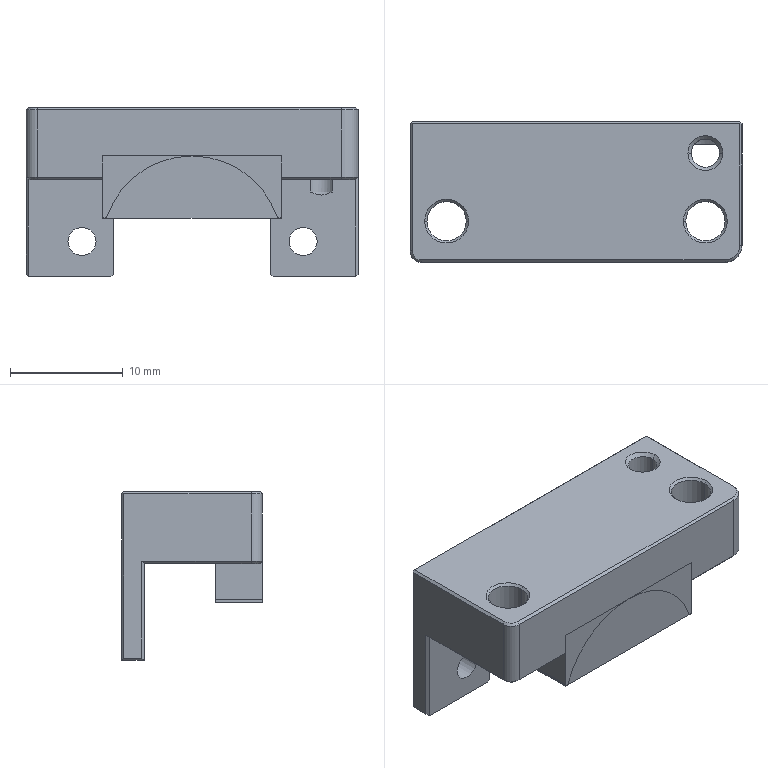Part | 2 solids | 71 faces | box 29.5 x 12.5 x 15 mm | volume 2665 mm3 | plane 41 | cylinder 15 | cone 15 | commonest cylinder face diameters 2.5 x6 3.5 x4 0.4 x2 2 x1 3 x1 16 x1